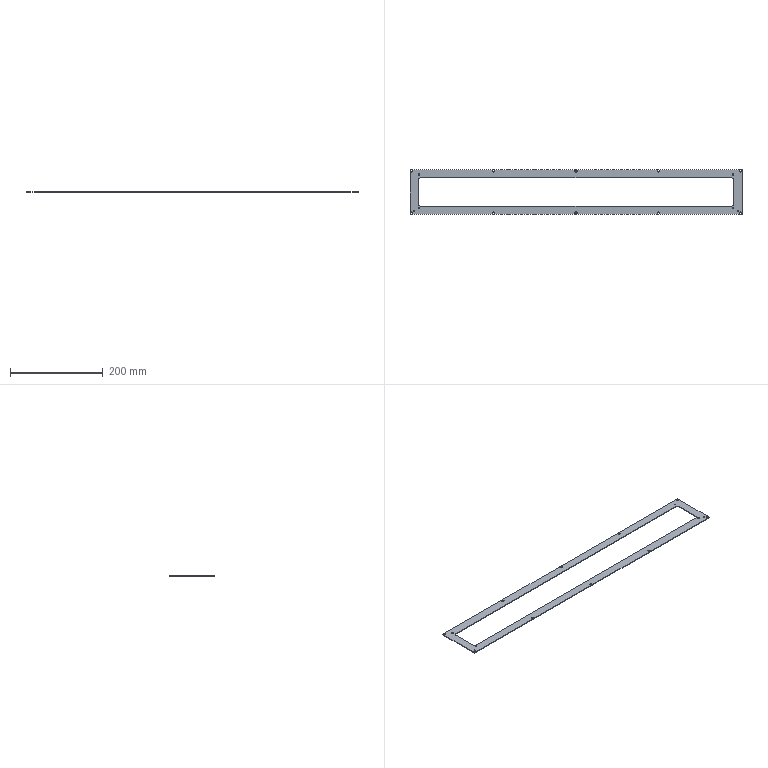Part | STEP file | Trunking Cover 2 Spacer Plate | 1 solid | 46 faces | box 716 x 97.011 x 1.5 mm | volume 41639 mm3 | cylinder 36 | plane 10 | commonest cylinder face diameters 5 x20 3.2 x8 2 x4 10 x4